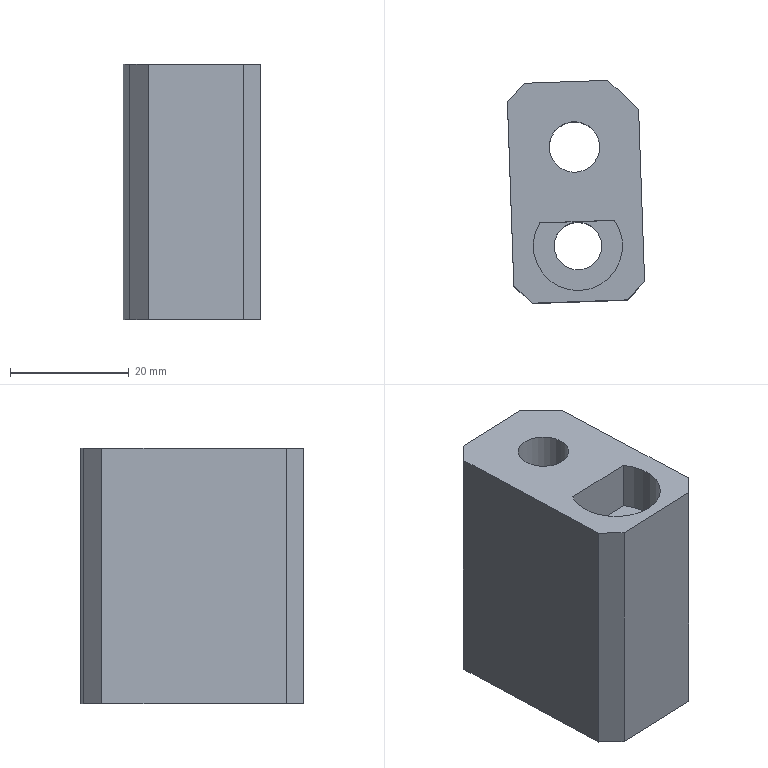Part | NX | features PH-9 2 | 1 solid | 17 faces | box 23.068 x 37.466 x 43 mm | volume 27290 mm3 | plane 13 | cylinder 4 | commonest cylinder face diameters 8.001 x1 8.5 x1 14.5 x1 15 x1
STEP:
#1=CARTESIAN_POINT('',(3189.932,-792.749,945.716));
#2=VERTEX_POINT('',#1);
#3=CARTESIAN_POINT('',(3185.685,-792.898,945.716));
#4=DIRECTION('',(0.,0.,1.));
#5=DIRECTION('',(0.9994,0.0349,0.));
#6=AXIS2_PLACEMENT_3D('',#3,#4,#5);
#7=CIRCLE('',#6,4.25);
#8=EDGE_CURVE('',#2,#2,#7,.T.);
#9=ORIENTED_EDGE('',*,*,#8,.F.);
#10=EDGE_LOOP('',(#9));
#11=FACE_BOUND('',#10,.T.);
#12=CARTESIAN_POINT('',(3196.469,-786.517,945.716));
#13=VERTEX_POINT('',#12);
#14=CARTESIAN_POINT('',(3197.481,-815.5,945.716));
#15=VERTEX_POINT('',#14);
#16=CARTESIAN_POINT('',(3196.922,-799.509,945.716));
#17=DIRECTION('',(0.0349,-0.9994,0.));
#18=VECTOR('',#17,1000.);
#19=LINE('',#16,#18);
#20=EDGE_CURVE('',#13,#15,#19,.T.);
#21=ORIENTED_EDGE('',*,*,#20,.F.);
#22=CARTESIAN_POINT('',(3191.297,-781.695,945.716));
#23=VERTEX_POINT('',#22);
#24=CARTESIAN_POINT('',(3197.503,-787.482,945.716));
#25=DIRECTION('',(0.7314,-0.682,0.));
#26=VECTOR('',#25,1000.);
#27=LINE('',#24,#26);
#28=EDGE_CURVE('',#13,#23,#27,.F.);
#29=ORIENTED_EDGE('',*,*,#28,.T.);
#30=CARTESIAN_POINT('',(3177.306,-782.183,945.716));
#31=VERTEX_POINT('',#30);
#32=CARTESIAN_POINT('',(3185.301,-781.904,945.716));
#33=DIRECTION('',(0.9994,0.0349,0.));
#34=VECTOR('',#33,1000.);
#35=LINE('',#32,#34);
#36=EDGE_CURVE('',#31,#23,#35,.T.);
#37=ORIENTED_EDGE('',*,*,#36,.F.);
#38=CARTESIAN_POINT('',(3174.412,-785.286,945.716));
#39=VERTEX_POINT('',#38);
#40=CARTESIAN_POINT('',(3172.483,-787.355,945.716));
#41=DIRECTION('',(0.682,0.7314,0.));
#42=VECTOR('',#41,1000.);
#43=LINE('',#40,#42);
#44=EDGE_CURVE('',#31,#39,#43,.F.);
#45=ORIENTED_EDGE('',*,*,#44,.T.);
#46=CARTESIAN_POINT('',(3175.494,-816.267,945.716));
#47=VERTEX_POINT('',#46);
#48=CARTESIAN_POINT('',(3174.936,-800.277,945.716));
#49=DIRECTION('',(-0.0349,0.9994,0.));
#50=VECTOR('',#49,1000.);
#51=LINE('',#48,#50);
#52=EDGE_CURVE('',#47,#39,#51,.T.);
#53=ORIENTED_EDGE('',*,*,#52,.F.);
#54=CARTESIAN_POINT('',(3178.597,-819.161,945.716));
#55=VERTEX_POINT('',#54);
#56=CARTESIAN_POINT('',(3172.908,-813.856,945.716));
#57=DIRECTION('',(-0.7314,0.682,0.));
#58=VECTOR('',#57,1000.);
#59=LINE('',#56,#58);
#60=EDGE_CURVE('',#47,#55,#59,.F.);
#61=ORIENTED_EDGE('',*,*,#60,.T.);
#62=CARTESIAN_POINT('',(3194.587,-818.603,945.716));
#63=VERTEX_POINT('',#62);
#64=CARTESIAN_POINT('',(3186.592,-818.882,945.716));
#65=DIRECTION('',(-0.9994,-0.0349,0.));
#66=VECTOR('',#65,1000.);
#67=LINE('',#64,#66);
#68=EDGE_CURVE('',#63,#55,#67,.T.);
#69=ORIENTED_EDGE('',*,*,#68,.F.);
#70=CARTESIAN_POINT('',(3199.892,-812.914,945.716));
#71=DIRECTION('',(-0.682,-0.7314,0.));
#72=VECTOR('',#71,1000.);
#73=LINE('',#70,#72);
#74=EDGE_CURVE('',#63,#15,#73,.F.);
#75=ORIENTED_EDGE('',*,*,#74,.T.);
#76=EDGE_LOOP('',(#21,#29,#37,#45,#53,#61,#69,#75));
#77=FACE_BOUND('',#76,.T.);
#78=CARTESIAN_POINT('',(3179.846,-805.66,945.716));
#79=VERTEX_POINT('',#78);
#80=CARTESIAN_POINT('',(3192.399,-805.221,945.716));
#81=VERTEX_POINT('',#80);
#82=CARTESIAN_POINT('',(3186.266,-809.538,945.716));
#83=DIRECTION('',(0.,0.,1.));
#84=DIRECTION('',(1.,0.,0.));
#85=AXIS2_PLACEMENT_3D('',#82,#83,#84);
#86=CIRCLE('',#85,7.5);
#87=EDGE_CURVE('',#79,#81,#86,.T.);
#88=ORIENTED_EDGE('',*,*,#87,.F.);
#89=CARTESIAN_POINT('',(3186.123,-805.44,945.716));
#90=DIRECTION('',(0.9994,0.0349,0.));
#91=VECTOR('',#90,1000.);
#92=LINE('',#89,#91);
#93=EDGE_CURVE('',#79,#81,#92,.T.);
#94=ORIENTED_EDGE('',*,*,#93,.T.);
#95=EDGE_LOOP('',(#88,#94));
#96=FACE_BOUND('',#95,.T.);
#97=CARTESIAN_POINT('',(3185.929,-799.893,945.716));
#98=DIRECTION('',(0.,0.,1.));
#99=DIRECTION('',(0.9994,0.0349,0.));
#100=AXIS2_PLACEMENT_3D('',#97,#98,#99);
#101=PLANE('',#100);
#102=ADVANCED_FACE('',(#11,#77,#96),#101,.T.);
#103=CARTESIAN_POINT('',(3178.597,-819.161,902.716));
#104=VERTEX_POINT('',#103);
#105=CARTESIAN_POINT('',(3194.587,-818.603,902.716));
#106=VERTEX_POINT('',#105);
#107=CARTESIAN_POINT('',(3186.592,-818.882,902.716));
#108=DIRECTION('',(0.9994,0.0349,0.));
#109=VECTOR('',#108,1000.);
#110=LINE('',#107,#109);
#111=EDGE_CURVE('',#104,#106,#110,.T.);
#112=ORIENTED_EDGE('',*,*,#111,.T.);
#113=CARTESIAN_POINT('',(3194.587,-818.603,920.716));
#114=DIRECTION('',(0.,0.,-1.));
#115=VECTOR('',#114,1000.);
#116=LINE('',#113,#115);
#117=EDGE_CURVE('',#106,#63,#116,.F.);
#118=ORIENTED_EDGE('',*,*,#117,.T.);
#119=ORIENTED_EDGE('',*,*,#68,.T.);
#120=CARTESIAN_POINT('',(3178.597,-819.161,920.716));
#121=DIRECTION('',(0.,0.,1.));
#122=VECTOR('',#121,1000.);
#123=LINE('',#120,#122);
#124=EDGE_CURVE('',#55,#104,#123,.F.);
#125=ORIENTED_EDGE('',*,*,#124,.T.);
#126=EDGE_LOOP('',(#112,#118,#119,#125));
#127=FACE_BOUND('',#126,.T.);
#128=CARTESIAN_POINT('',(3186.592,-818.882,920.716));
#129=DIRECTION('',(0.0349,-0.9994,0.));
#130=DIRECTION('',(0.,0.,-1.));
#131=AXIS2_PLACEMENT_3D('',#128,#129,#130);
#132=PLANE('',#131);
#133=ADVANCED_FACE('',(#127),#132,.T.);
#134=ORIENTED_EDGE('',*,*,#52,.T.);
#135=CARTESIAN_POINT('',(3174.412,-785.286,902.716));
#136=VERTEX_POINT('',#135);
#137=CARTESIAN_POINT('',(3174.412,-785.286,920.716));
#138=DIRECTION('',(0.,0.,-1.));
#139=VECTOR('',#138,1000.);
#140=LINE('',#137,#139);
#141=EDGE_CURVE('',#39,#136,#140,.T.);
#142=ORIENTED_EDGE('',*,*,#141,.T.);
#143=CARTESIAN_POINT('',(3175.494,-816.267,902.716));
#144=VERTEX_POINT('',#143);
#145=CARTESIAN_POINT('',(3174.936,-800.277,902.716));
#146=DIRECTION('',(0.0349,-0.9994,0.));
#147=VECTOR('',#146,1000.);
#148=LINE('',#145,#147);
#149=EDGE_CURVE('',#136,#144,#148,.T.);
#150=ORIENTED_EDGE('',*,*,#149,.T.);
#151=CARTESIAN_POINT('',(3175.494,-816.267,920.716));
#152=DIRECTION('',(0.,0.,-1.));
#153=VECTOR('',#152,1000.);
#154=LINE('',#151,#153);
#155=EDGE_CURVE('',#144,#47,#154,.F.);
#156=ORIENTED_EDGE('',*,*,#155,.T.);
#157=EDGE_LOOP('',(#134,#142,#150,#156));
#158=FACE_BOUND('',#157,.T.);
#159=CARTESIAN_POINT('',(3174.936,-800.277,920.716));
#160=DIRECTION('',(-0.9994,-0.0349,0.));
#161=DIRECTION('',(0.,0.,1.));
#162=AXIS2_PLACEMENT_3D('',#159,#160,#161);
#163=PLANE('',#162);
#164=ADVANCED_FACE('',(#158),#163,.T.);
#165=ORIENTED_EDGE('',*,*,#36,.T.);
#166=CARTESIAN_POINT('',(3191.297,-781.695,902.716));
#167=VERTEX_POINT('',#166);
#168=CARTESIAN_POINT('',(3191.297,-781.695,920.716));
#169=DIRECTION('',(0.,0.,-1.));
#170=VECTOR('',#169,1000.);
#171=LINE('',#168,#170);
#172=EDGE_CURVE('',#23,#167,#171,.T.);
#173=ORIENTED_EDGE('',*,*,#172,.T.);
#174=CARTESIAN_POINT('',(3177.306,-782.183,902.716));
#175=VERTEX_POINT('',#174);
#176=CARTESIAN_POINT('',(3185.301,-781.904,902.716));
#177=DIRECTION('',(-0.9994,-0.0349,0.));
#178=VECTOR('',#177,1000.);
#179=LINE('',#176,#178);
#180=EDGE_CURVE('',#167,#175,#179,.T.);
#181=ORIENTED_EDGE('',*,*,#180,.T.);
#182=CARTESIAN_POINT('',(3177.306,-782.183,920.716));
#183=DIRECTION('',(0.,0.,1.));
#184=VECTOR('',#183,1000.);
#185=LINE('',#182,#184);
#186=EDGE_CURVE('',#175,#31,#185,.T.);
#187=ORIENTED_EDGE('',*,*,#186,.T.);
#188=EDGE_LOOP('',(#165,#173,#181,#187));
#189=FACE_BOUND('',#188,.T.);
#190=CARTESIAN_POINT('',(3185.301,-781.904,920.716));
#191=DIRECTION('',(-0.0349,0.9994,0.));
#192=DIRECTION('',(0.,0.,1.));
#193=AXIS2_PLACEMENT_3D('',#190,#191,#192);
#194=PLANE('',#193);
#195=ADVANCED_FACE('',(#189),#194,.T.);
#196=CARTESIAN_POINT('',(3182.265,-809.538,902.716));
#197=VERTEX_POINT('',#196);
#198=CARTESIAN_POINT('',(3186.266,-809.538,902.716));
#199=DIRECTION('',(0.,0.,-1.));
#200=DIRECTION('',(-1.,0.,0.));
#201=AXIS2_PLACEMENT_3D('',#198,#199,#200);
#202=CIRCLE('',#201,4.);
#203=EDGE_CURVE('',#197,#197,#202,.T.);
#204=ORIENTED_EDGE('',*,*,#203,.F.);
#205=EDGE_LOOP('',(#204));
#206=FACE_BOUND('',#205,.T.);
#207=CARTESIAN_POINT('',(3178.435,-792.898,902.716));
#208=VERTEX_POINT('',#207);
#209=CARTESIAN_POINT('',(3185.685,-792.898,902.716));
#210=DIRECTION('',(0.,0.,-1.));
#211=DIRECTION('',(-1.,0.,0.));
#212=AXIS2_PLACEMENT_3D('',#209,#210,#211);
#213=CIRCLE('',#212,7.25);
#214=EDGE_CURVE('',#208,#208,#213,.F.);
#215=ORIENTED_EDGE('',*,*,#214,.T.);
#216=EDGE_LOOP('',(#215));
#217=FACE_BOUND('',#216,.T.);
#218=ORIENTED_EDGE('',*,*,#180,.F.);
#219=CARTESIAN_POINT('',(3196.469,-786.517,902.716));
#220=VERTEX_POINT('',#219);
#221=CARTESIAN_POINT('',(3197.503,-787.482,902.716));
#222=DIRECTION('',(-0.7314,0.682,0.));
#223=VECTOR('',#222,1000.);
#224=LINE('',#221,#223);
#225=EDGE_CURVE('',#167,#220,#224,.F.);
#226=ORIENTED_EDGE('',*,*,#225,.T.);
#227=CARTESIAN_POINT('',(3197.481,-815.5,902.716));
#228=VERTEX_POINT('',#227);
#229=CARTESIAN_POINT('',(3196.922,-799.509,902.716));
#230=DIRECTION('',(-0.0349,0.9994,0.));
#231=VECTOR('',#230,1000.);
#232=LINE('',#229,#231);
#233=EDGE_CURVE('',#228,#220,#232,.T.);
#234=ORIENTED_EDGE('',*,*,#233,.F.);
#235=CARTESIAN_POINT('',(3199.892,-812.914,902.716));
#236=DIRECTION('',(0.682,0.7314,0.));
#237=VECTOR('',#236,1000.);
#238=LINE('',#235,#237);
#239=EDGE_CURVE('',#228,#106,#238,.F.);
#240=ORIENTED_EDGE('',*,*,#239,.T.);
#241=ORIENTED_EDGE('',*,*,#111,.F.);
#242=CARTESIAN_POINT('',(3172.908,-813.856,902.716));
#243=DIRECTION('',(0.7314,-0.682,0.));
#244=VECTOR('',#243,1000.);
#245=LINE('',#242,#244);
#246=EDGE_CURVE('',#104,#144,#245,.F.);
#247=ORIENTED_EDGE('',*,*,#246,.T.);
#248=ORIENTED_EDGE('',*,*,#149,.F.);
#249=CARTESIAN_POINT('',(3172.483,-787.355,902.716));
#250=DIRECTION('',(-0.682,-0.7314,0.));
#251=VECTOR('',#250,1000.);
#252=LINE('',#249,#251);
#253=EDGE_CURVE('',#136,#175,#252,.F.);
#254=ORIENTED_EDGE('',*,*,#253,.T.);
#255=EDGE_LOOP('',(#218,#226,#234,#240,#241,#247,#248,#254));
#256=FACE_BOUND('',#255,.T.);
#257=CARTESIAN_POINT('',(3185.929,-799.893,902.716));
#258=DIRECTION('',(0.,0.,-1.));
#259=DIRECTION('',(-0.9994,-0.0349,0.));
#260=AXIS2_PLACEMENT_3D('',#257,#258,#259);
#261=PLANE('',#260);
#262=ADVANCED_FACE('',(#206,#217,#256),#261,.T.);
#263=ORIENTED_EDGE('',*,*,#233,.T.);
#264=CARTESIAN_POINT('',(3196.469,-786.517,920.716));
#265=DIRECTION('',(0.,0.,1.));
#266=VECTOR('',#265,1000.);
#267=LINE('',#264,#266);
#268=EDGE_CURVE('',#220,#13,#267,.T.);
#269=ORIENTED_EDGE('',*,*,#268,.T.);
#270=ORIENTED_EDGE('',*,*,#20,.T.);
#271=CARTESIAN_POINT('',(3197.481,-815.5,920.716));
#272=DIRECTION('',(0.,0.,1.));
#273=VECTOR('',#272,1000.);
#274=LINE('',#271,#273);
#275=EDGE_CURVE('',#15,#228,#274,.F.);
#276=ORIENTED_EDGE('',*,*,#275,.T.);
#277=EDGE_LOOP('',(#263,#269,#270,#276));
#278=FACE_BOUND('',#277,.T.);
#279=CARTESIAN_POINT('',(3196.922,-799.509,920.716));
#280=DIRECTION('',(0.9994,0.0349,0.));
#281=DIRECTION('',(0.,0.,-1.));
#282=AXIS2_PLACEMENT_3D('',#279,#280,#281);
#283=PLANE('',#282);
#284=ADVANCED_FACE('',(#278),#283,.T.);
#285=ORIENTED_EDGE('',*,*,#239,.F.);
#286=ORIENTED_EDGE('',*,*,#275,.F.);
#287=ORIENTED_EDGE('',*,*,#74,.F.);
#288=ORIENTED_EDGE('',*,*,#117,.F.);
#289=EDGE_LOOP('',(#285,#286,#287,#288));
#290=FACE_BOUND('',#289,.T.);
#291=CARTESIAN_POINT('',(3194.587,-818.603,920.716));
#292=DIRECTION('',(-0.7314,0.682,0.));
#293=DIRECTION('',(-0.682,-0.7314,0.));
#294=AXIS2_PLACEMENT_3D('',#291,#292,#293);
#295=PLANE('',#294);
#296=ADVANCED_FACE('',(#290),#295,.F.);
#297=ORIENTED_EDGE('',*,*,#246,.F.);
#298=ORIENTED_EDGE('',*,*,#124,.F.);
#299=ORIENTED_EDGE('',*,*,#60,.F.);
#300=ORIENTED_EDGE('',*,*,#155,.F.);
#301=EDGE_LOOP('',(#297,#298,#299,#300));
#302=FACE_BOUND('',#301,.T.);
#303=CARTESIAN_POINT('',(3175.494,-816.267,920.716));
#304=DIRECTION('',(0.682,0.7314,0.));
#305=DIRECTION('',(-0.7314,0.682,0.));
#306=AXIS2_PLACEMENT_3D('',#303,#304,#305);
#307=PLANE('',#306);
#308=ADVANCED_FACE('',(#302),#307,.F.);
#309=ORIENTED_EDGE('',*,*,#253,.F.);
#310=ORIENTED_EDGE('',*,*,#141,.F.);
#311=ORIENTED_EDGE('',*,*,#44,.F.);
#312=ORIENTED_EDGE('',*,*,#186,.F.);
#313=EDGE_LOOP('',(#309,#310,#311,#312));
#314=FACE_BOUND('',#313,.T.);
#315=CARTESIAN_POINT('',(3177.306,-782.183,920.716));
#316=DIRECTION('',(0.7314,-0.682,0.));
#317=DIRECTION('',(0.682,0.7314,0.));
#318=AXIS2_PLACEMENT_3D('',#315,#316,#317);
#319=PLANE('',#318);
#320=ADVANCED_FACE('',(#314),#319,.F.);
#321=CARTESIAN_POINT('',(3189.935,-792.898,913.716));
#322=VERTEX_POINT('',#321);
#323=CARTESIAN_POINT('',(3185.685,-792.898,913.716));
#324=DIRECTION('',(0.,0.,1.));
#325=DIRECTION('',(1.,0.,0.));
#326=AXIS2_PLACEMENT_3D('',#323,#324,#325);
#327=CIRCLE('',#326,4.25);
#328=EDGE_CURVE('',#322,#322,#327,.T.);
#329=ORIENTED_EDGE('',*,*,#328,.T.);
#330=EDGE_LOOP('',(#329));
#331=FACE_BOUND('',#330,.T.);
#332=CARTESIAN_POINT('',(3192.935,-792.898,913.716));
#333=VERTEX_POINT('',#332);
#334=CARTESIAN_POINT('',(3185.685,-792.898,913.716));
#335=DIRECTION('',(0.,0.,1.));
#336=DIRECTION('',(1.,0.,0.));
#337=AXIS2_PLACEMENT_3D('',#334,#335,#336);
#338=CIRCLE('',#337,7.25);
#339=EDGE_CURVE('',#333,#333,#338,.T.);
#340=ORIENTED_EDGE('',*,*,#339,.F.);
#341=EDGE_LOOP('',(#340));
#342=FACE_BOUND('',#341,.T.);
#343=CARTESIAN_POINT('',(3185.685,-792.898,913.716));
#344=DIRECTION('',(0.,0.,1.));
#345=DIRECTION('',(0.9994,0.0349,0.));
#346=AXIS2_PLACEMENT_3D('',#343,#344,#345);
#347=PLANE('',#346);
#348=ADVANCED_FACE('',(#331,#342),#347,.F.);
#349=ORIENTED_EDGE('',*,*,#214,.F.);
#350=EDGE_LOOP('',(#349));
#351=FACE_BOUND('',#350,.T.);
#352=ORIENTED_EDGE('',*,*,#339,.T.);
#353=EDGE_LOOP('',(#352));
#354=FACE_BOUND('',#353,.T.);
#355=CARTESIAN_POINT('',(3185.685,-792.898,931.716));
#356=DIRECTION('',(0.,0.,-1.));
#357=DIRECTION('',(0.9994,0.0349,0.));
#358=AXIS2_PLACEMENT_3D('',#355,#356,#357);
#359=CYLINDRICAL_SURFACE('',#358,7.25);
#360=ADVANCED_FACE('',(#351,#354),#359,.F.);
#361=ORIENTED_EDGE('',*,*,#8,.T.);
#362=EDGE_LOOP('',(#361));
#363=FACE_BOUND('',#362,.T.);
#364=ORIENTED_EDGE('',*,*,#328,.F.);
#365=EDGE_LOOP('',(#364));
#366=FACE_BOUND('',#365,.T.);
#367=CARTESIAN_POINT('',(3185.685,-792.898,946.716));
#368=DIRECTION('',(0.,0.,-1.));
#369=DIRECTION('',(0.9994,0.0349,0.));
#370=AXIS2_PLACEMENT_3D('',#367,#368,#369);
#371=CYLINDRICAL_SURFACE('',#370,4.25);
#372=ADVANCED_FACE('',(#363,#366),#371,.F.);
#373=CARTESIAN_POINT('',(3182.265,-809.538,937.416));
#374=VERTEX_POINT('',#373);
#375=CARTESIAN_POINT('',(3186.266,-809.538,937.416));
#376=DIRECTION('',(0.,0.,1.));
#377=DIRECTION('',(-1.,0.,0.));
#378=AXIS2_PLACEMENT_3D('',#375,#376,#377);
#379=CIRCLE('',#378,4.);
#380=EDGE_CURVE('',#374,#374,#379,.F.);
#381=ORIENTED_EDGE('',*,*,#380,.T.);
#382=EDGE_LOOP('',(#381));
#383=FACE_BOUND('',#382,.T.);
#384=CARTESIAN_POINT('',(3192.399,-805.221,937.416));
#385=VERTEX_POINT('',#384);
#386=CARTESIAN_POINT('',(3179.846,-805.66,937.416));
#387=VERTEX_POINT('',#386);
#388=CARTESIAN_POINT('',(3186.123,-805.44,937.416));
#389=DIRECTION('',(-0.9994,-0.0349,0.));
#390=VECTOR('',#389,1000.);
#391=LINE('',#388,#390);
#392=EDGE_CURVE('',#385,#387,#391,.T.);
#393=ORIENTED_EDGE('',*,*,#392,.T.);
#394=CARTESIAN_POINT('',(3186.266,-809.538,937.416));
#395=DIRECTION('',(0.,0.,-1.));
#396=DIRECTION('',(1.,0.,0.));
#397=AXIS2_PLACEMENT_3D('',#394,#395,#396);
#398=CIRCLE('',#397,7.5);
#399=EDGE_CURVE('',#385,#387,#398,.T.);
#400=ORIENTED_EDGE('',*,*,#399,.F.);
#401=EDGE_LOOP('',(#393,#400));
#402=FACE_BOUND('',#401,.T.);
#403=CARTESIAN_POINT('',(3186.266,-809.538,937.416));
#404=DIRECTION('',(0.,0.,-1.));
#405=DIRECTION('',(-1.,0.,0.));
#406=AXIS2_PLACEMENT_3D('',#403,#404,#405);
#407=PLANE('',#406);
#408=ADVANCED_FACE('',(#383,#402),#407,.F.);
#409=ORIENTED_EDGE('',*,*,#28,.F.);
#410=ORIENTED_EDGE('',*,*,#268,.F.);
#411=ORIENTED_EDGE('',*,*,#225,.F.);
#412=ORIENTED_EDGE('',*,*,#172,.F.);
#413=EDGE_LOOP('',(#409,#410,#411,#412));
#414=FACE_BOUND('',#413,.T.);
#415=CARTESIAN_POINT('',(3191.297,-781.695,920.716));
#416=DIRECTION('',(-0.682,-0.7314,0.));
#417=DIRECTION('',(0.,0.,-1.));
#418=AXIS2_PLACEMENT_3D('',#415,#416,#417);
#419=PLANE('',#418);
#420=ADVANCED_FACE('',(#414),#419,.F.);
#421=ORIENTED_EDGE('',*,*,#93,.F.);
#422=CARTESIAN_POINT('',(3179.846,-805.66,945.716));
#423=DIRECTION('',(0.,0.,-1.));
#424=VECTOR('',#423,1000.);
#425=LINE('',#422,#424);
#426=EDGE_CURVE('',#387,#79,#425,.F.);
#427=ORIENTED_EDGE('',*,*,#426,.F.);
#428=ORIENTED_EDGE('',*,*,#392,.F.);
#429=CARTESIAN_POINT('',(3192.399,-805.221,945.716));
#430=DIRECTION('',(0.,0.,-1.));
#431=VECTOR('',#430,1000.);
#432=LINE('',#429,#431);
#433=EDGE_CURVE('',#81,#385,#432,.T.);
#434=ORIENTED_EDGE('',*,*,#433,.F.);
#435=EDGE_LOOP('',(#421,#427,#428,#434));
#436=FACE_BOUND('',#435,.T.);
#437=CARTESIAN_POINT('',(3186.123,-805.44,960.966));
#438=DIRECTION('',(-0.0349,0.9994,0.));
#439=DIRECTION('',(0.9994,0.0349,0.));
#440=AXIS2_PLACEMENT_3D('',#437,#438,#439);
#441=PLANE('',#440);
#442=ADVANCED_FACE('',(#436),#441,.F.);
#443=ORIENTED_EDGE('',*,*,#399,.T.);
#444=ORIENTED_EDGE('',*,*,#426,.T.);
#445=ORIENTED_EDGE('',*,*,#87,.T.);
#446=ORIENTED_EDGE('',*,*,#433,.T.);
#447=EDGE_LOOP('',(#443,#444,#445,#446));
#448=FACE_BOUND('',#447,.T.);
#449=CARTESIAN_POINT('',(3186.266,-809.538,945.716));
#450=DIRECTION('',(0.,0.,-1.));
#451=DIRECTION('',(1.,0.,0.));
#452=AXIS2_PLACEMENT_3D('',#449,#450,#451);
#453=CYLINDRICAL_SURFACE('',#452,7.5);
#454=ADVANCED_FACE('',(#448),#453,.F.);
#455=ORIENTED_EDGE('',*,*,#203,.T.);
#456=EDGE_LOOP('',(#455));
#457=FACE_BOUND('',#456,.T.);
#458=ORIENTED_EDGE('',*,*,#380,.F.);
#459=EDGE_LOOP('',(#458));
#460=FACE_BOUND('',#459,.T.);
#461=CARTESIAN_POINT('',(3186.266,-809.538,945.716));
#462=DIRECTION('',(0.,0.,-1.));
#463=DIRECTION('',(1.,0.,0.));
#464=AXIS2_PLACEMENT_3D('',#461,#462,#463);
#465=CYLINDRICAL_SURFACE('',#464,4.);
#466=ADVANCED_FACE('',(#457,#460),#465,.F.);
#467=CLOSED_SHELL('',(#102,#133,#164,#195,#262,#284,#296,#308,#320,#348,#360,#372,#408,#420,#442,#454,#466));
#468=MANIFOLD_SOLID_BREP('',#467);
#469=(LENGTH_UNIT()NAMED_UNIT(*)SI_UNIT(.MILLI.,.METRE.));
#470=UNCERTAINTY_MEASURE_WITH_UNIT(LENGTH_MEASURE(0.00001),#469,'','');
#471=(NAMED_UNIT(*)PLANE_ANGLE_UNIT()SI_UNIT($,.RADIAN.));
#472=(NAMED_UNIT(*)SI_UNIT($,.STERADIAN.)SOLID_ANGLE_UNIT());
#473=(GEOMETRIC_REPRESENTATION_CONTEXT(3)GLOBAL_UNCERTAINTY_ASSIGNED_CONTEXT((#470))GLOBAL_UNIT_ASSIGNED_CONTEXT((#469,#471,#472))REPRESENTATION_CONTEXT('',''));
#474=ADVANCED_BREP_SHAPE_REPRESENTATION('',(#468),#473);